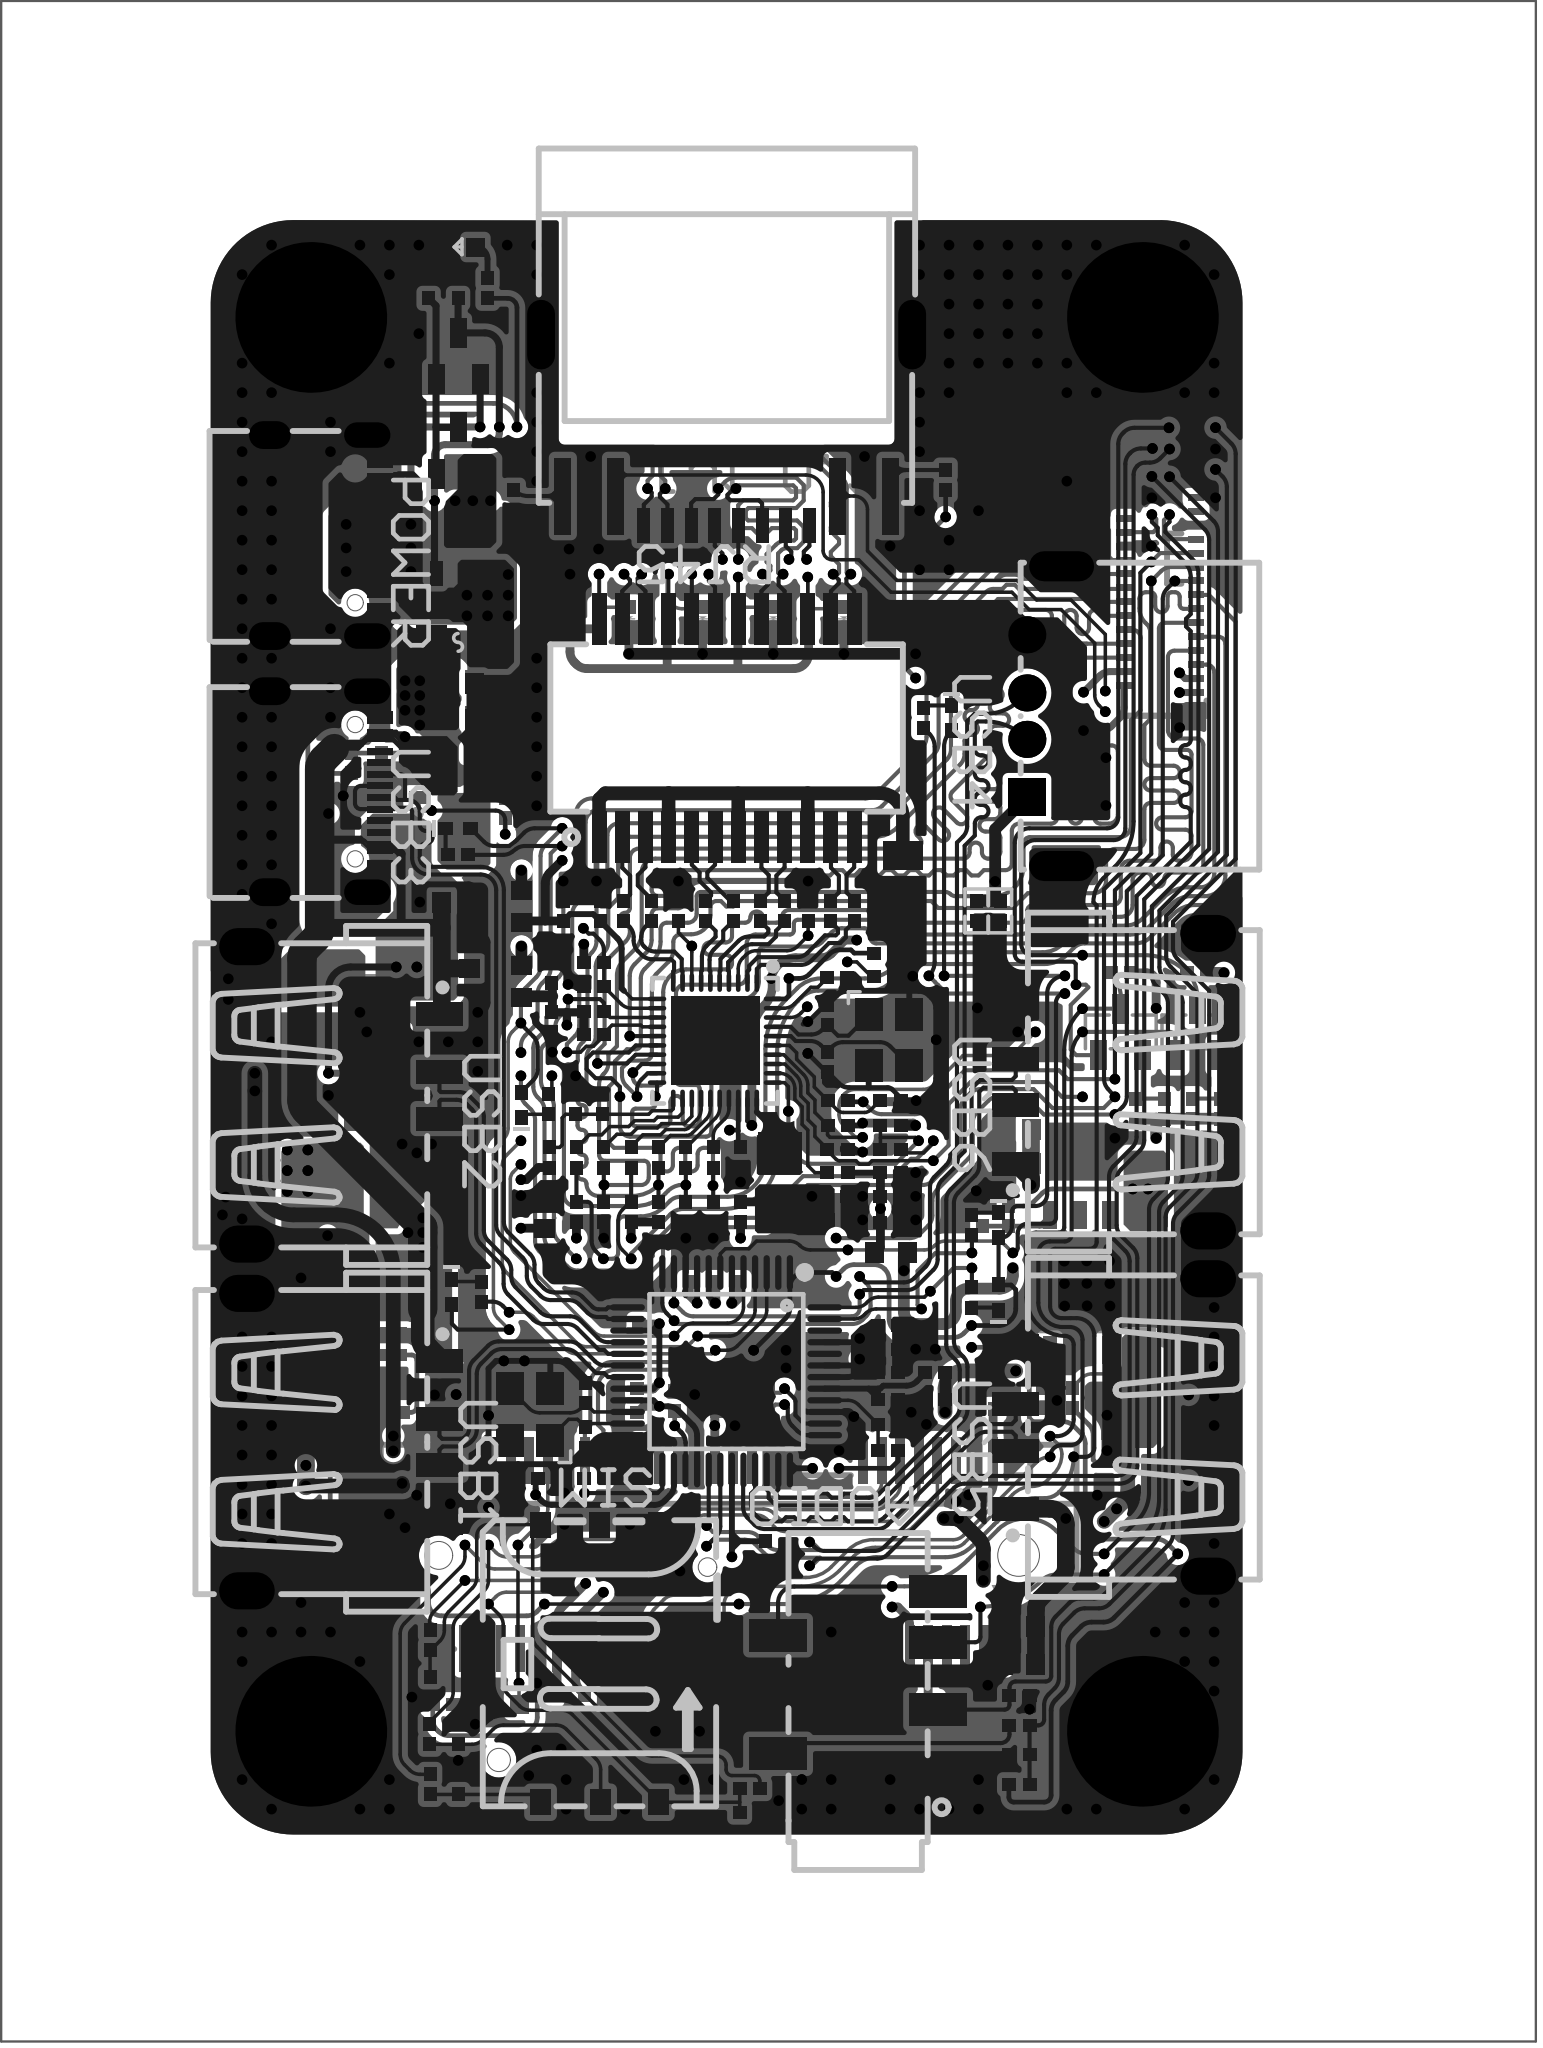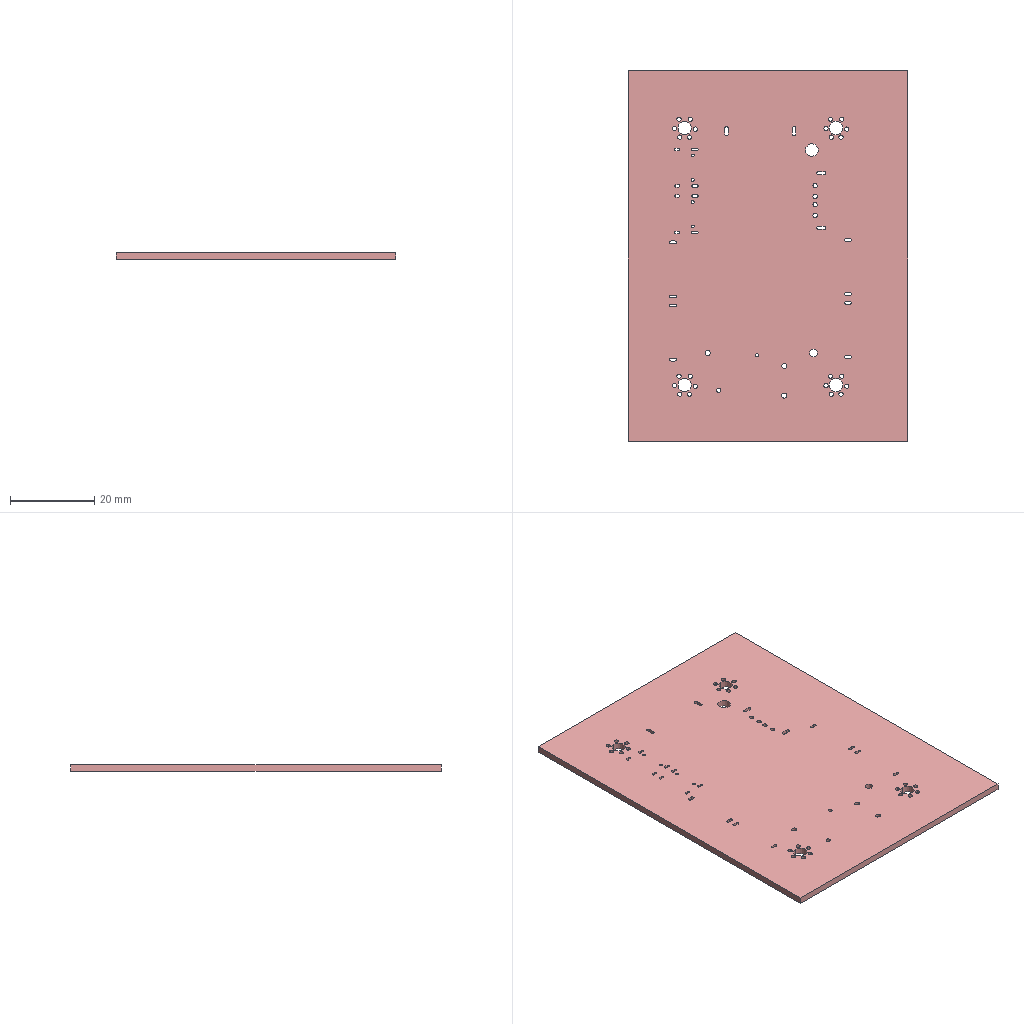Circuit board layout | Altium Designer | box 66.2 x 87.8 x 1.6 mm
Layer stack:
# Altium Designer layer stack of  (unit mm; dielectric type: 0 none, 1 core, 2 prepreg, 3 surface material)
index,name,kind,layer,copper_thickness_mm,dielectric_type,dielectric_thickness_mm,dielectric_material,dielectric_constant
0,Top Paste Mask Layer,other,,,,,,
1,Top Silkscreen Layer,other,,,,,,
2,Top Solder Mask Layer,dielectric,,,3,0,,0
3,Top Layer,copper,Top Layer,0.035,,,,
4,Dielectric1,dielectric,,,3,0.2104,7628 RC49% 8.6mil,0
5,GND,copper,GND,0.0152,,,,
6,Dielectric2,dielectric,,,3,1.065,1.1mm H/HOZ \u00BA\u00AC\u00CD\u00AD,0
7,VCC,copper,VCC,0.0152,,,,
8,Dielectric3,dielectric,,,3,0.2104,7628 RC49% 8.6mil,0
9,Bottom Layer,copper,Bottom Layer,0.035,,,,
10,Bottom Solder Mask Layer,dielectric,,,3,0,,0
11,Bottom Silkscreen Layer,other,,,,,,
12,Bottom Paste Mask Layer,other,,,,,,
# drill layer pairs: low layer,high layer
drill_pair,Top Layer,Bottom Layer
Part placement:
Designator,Comment,Layer,Footprint,Center-X(mm),Center-Y(mm),Rotation
R67,10kΩ,BottomLayer,R0402,118.125,115.839,0
R66,4.7kΩ,BottomLayer,R0402,118.76,109.997,90
R72,4.7kΩ,BottomLayer,R0402,121.203,109.997,270
FPC1,AFE03-S39FMA-1H,BottomLayer,fpc-smd_p0.30-39p_fgs-xj-h1.0,119.819,133.606,270
R70,10kΩ,BottomLayer,R0402,88.892,84.358,180
Q1,CJ2301 S1,TopLayer,SOT-23-3_L3.0-W1.7-P0.95-LS2.9-BR,89.55,134.127,270
C2,100nF,TopLayer,r0603,89.55,126.761,180
Q2,MMBT5401,TopLayer,SOT-23-3_L2.9-W1.3-P1.90-LS2.4-BR,89.55,138.315,270
Q3,MMBT5401,TopLayer,SOT-23-3_L2.9-W1.3-P1.90-LS2.4-BR,89.55,142.382,270
R6,50kΩ,TopLayer,R0402,89.55,145.303,270
R5,10kΩ,TopLayer,R0402,88.28,145.303,270
C1,10uF,TopLayer,r0603,89.55,128.285,180
F1,BSMD0805L-200,TopLayer,F0805,89.55,130.063,180
U1,MD7672B50SF4,BottomLayer,ESOP-8_L4.9-W3.9-P1.27-LS6.0-BL-EP,116.982,102.504,180
C3,4.7uF,BottomLayer,C0603,118.252,107.584,0
C4,4.7uF,BottomLayer,C0603,117.998,97.678,0
R74,10kΩ,TopLayer,R0402,113.758,80.914,180
R1,220kΩ,BottomLayer,R0402,116.043,97.551,270
R2,15kΩ,BottomLayer,R0402,113.299,105.373,90
R3,10kΩ,BottomLayer,R0402,112.156,105.373,270
R4,50kΩ,BottomLayer,R0402,114.747,97.551,90
U2,SY8113BADC,BottomLayer,TSOT-23-6_L2.9-W1.6-P0.95-LS2.8-BR,89.042,124.348,180
C8,100nF,BottomLayer,r0603,89.548,128.412,180
C6,100nF,BottomLayer,R0402,91.582,122.951,270
C9,22pF,BottomLayer,R0402,84.96,124.856,270
R8,232kΩ,BottomLayer,R0402,83.708,124.856,270
LED1,19-217/GHC-YR1S2/3T,TopLayer,LED0603-RD,89.5,147.075,0
R11,50kΩ,BottomLayer,R0402,86.248,124.856,90
C10,22uF,BottomLayer,r0603,89.548,117.744,180
C11,100nF,BottomLayer,r0603,89.548,119.268,180
C7,10uF,BottomLayer,r0603,89.548,126.888,180
R7,15kΩ,BottomLayer,R0402,91.582,124.856,270
R9,10kΩ,BottomLayer,R0402,91.582,126.761,270
R10,4.7kΩ,TopLayer,R0402,90.82,145.303,270
U4,RTL8211F-CG,TopLayer,WQFN-40_L5.0-W5.0-P0.4-BL-EP,100.629,112.918,180
L4,CBM160808U121T,TopLayer,L0603,92.281,115.465,90
Q4,SS8050,BottomLayer,SOT-23-3_L2.9-W1.3-P1.90-LS2.4-BR,118.125,113.299,270
L5,CBM160808U121T,TopLayer,L0603,108.218,103.787,0
L6,CBM160808U121T,TopLayer,L0603,92.281,118.697,90
R36,4.7kΩ,TopLayer,R0402,108.194,109.273,0
R33,0Ω,TopLayer,R0402,108.194,108.257,0
R19,4.7kΩ,TopLayer,R0402,105.912,109.273,0
R17,4.7kΩ,TopLayer,R0402,105.909,108.257,0
R14,4.7kΩ,TopLayer,R0402,105.911,107.241,0
Q5,SS8050,BottomLayer,SOT-23-3_L2.9-W1.3-P1.90-LS2.4-BR,121.427,113.299,270
R49,0Ω,TopLayer,R0402,93.474,107.895,270
U6,SMTWE2050MTJ,BottomLayer,SMD_BD4.4-L4.4-D2.8,113.317,138.831,180
R18,4.7kΩ,TopLayer,R0402,94.654,105.552,90
R16,4.7kΩ,TopLayer,R0402,97.012,105.552,90
R13,4.7kΩ,TopLayer,R0402,98.191,105.552,90
R21,4.7kΩ,TopLayer,R0402,95.405,114.188,0
R20,4.7kΩ,TopLayer,R0402,95.405,113.191,0
R30,4.7kΩ,TopLayer,R0402,99.371,105.552,90
R26,4.7kΩ,TopLayer,R0402,100.55,105.552,90
R22,4.7kΩ,TopLayer,R0402,95.833,105.552,90
R42,10kΩ,TopLayer,R0402,95.405,116.284,180
R73,0Ω,TopLayer,R0402,113.758,84.724,0
R41,22Ω,TopLayer,R0402,100.55,107.895,270
R43,22Ω,TopLayer,R0402,99.371,107.895,270
R44,22Ω,TopLayer,R0402,98.191,107.895,270
R45,22Ω,TopLayer,R0402,97.012,107.895,270
R46,22Ω,TopLayer,R0402,95.833,107.895,270
R48,22Ω,TopLayer,R0402,94.654,107.895,270
R28,100Ω,TopLayer,R0402,105.915,110.365,0
R23,120Ω,TopLayer,R0402,108.194,110.365,0
USB2,TYPE-C 16PIN 2MD(073),TopLayer,USB-C-SMD_TYPE-C-6PIN-2MD-073,83.81,123.637,270
R15,2.49kΩ,TopLayer,R0402,105.908,115.648,0
R50,0Ω,TopLayer,R0402,101.729,105.552,270
L3,G2406S,TopLayer,SMD-24_L15.1-W7.1-P1.00-LS10.0-BL,101.129,126.38,0
RJ1,RC01812,TopLayer,RJ45-TH_RC01812,101.129,139.207,0
R51,510Ω,TopLayer,R0402,110.57,137.048,90
R47,510Ω,TopLayer,R0402,91.951,137.048,270
R37,75Ω,BottomLayer,R0402,104.663,131.079,90
R38,75Ω,BottomLayer,R0402,101.615,131.079,90
R39,75Ω,BottomLayer,R0402,98.567,131.079,90
R40,75Ω,BottomLayer,R0402,95.646,131.079,90
D1,KLXES15AAA1,BottomLayer,D0402-BI,96.916,131.075,270
D2,KLXES15AAA1,BottomLayer,D0402-BI,100.091,131.075,270
D3,KLXES15AAA1,BottomLayer,D0402-BI,103.139,131.075,270
D4,KLXES15AAA1,BottomLayer,D0402-BI,106.187,131.075,270
R24,0Ω,TopLayer,R0402,96.696,118.506,90
R25,0Ω,TopLayer,R0402,97.873,118.506,90
R27,0Ω,TopLayer,R0402,100.229,118.506,90
R29,0Ω,TopLayer,R0402,101.407,118.506,90
R31,0Ω,TopLayer,R0402,102.584,118.506,90
R32,0Ω,TopLayer,R0402,103.635,118.506,90
R34,0Ω,TopLayer,R0402,105.609,118.506,90
R35,0Ω,TopLayer,R0402,106.66,118.506,90
USB1,TYPE-C 16PIN 2MD(073),TopLayer,USB-C-SMD_TYPE-C-6PIN-2MD-073,83.81,134.66,270
U5,FE2.1-CQFP48A,TopLayer,LQFP-48_L7.0-W7.0-P0.50-LS9.0-BL,101.107,98.694,180
R71,10kΩ,BottomLayer,R0402,121.427,115.839,180
LED7,XL-1005UGC,TopLayer,LED0402-RD_GREEN,112.855,104.981,270
LED6,XL-1005UGC,TopLayer,LED0402-RD_GREEN,112.855,101.869,90
LED5,XL-1005UGC,TopLayer,LED0402-RD_GREEN,110.823,126.81,270
LED4,XL-1005UGC,TopLayer,LED0402-RD_GREEN,89.55,122.062,0
LED3,XL-1005UGC,TopLayer,LED0402-RD_GREEN,92.268,110.162,90
LED2,XL-1005UGC,TopLayer,LED0402-RD_GREEN,89.283,102.123,270
X2,12MHz,TopLayer,OSC-SMD_4P-L3.2-W2.5-BL,92.652,96.836,90
R58,2.7kΩ,BottomLayer,R0402,98.89,97.402,90
R60,47kΩ,TopLayer,R0402,110.133,98.63,0
R61,100kΩ,TopLayer,R0402,108.092,97.487,180
R59,100kΩ,TopLayer,R0402,108.092,95.28,0
USB4,AF 10.0 HC6.3,TopLayer,USB-A-TH_AF-10.0-HC6.3,114.823,126.888,90
C48,10uF,TopLayer,r0603,93.294,105.552,270
CN1,1775862-2,BottomLayer,PCI-SMD_1775862-2,101.218,90.62,0
R63,0Ω,TopLayer,R0402,88.335,83.073,270
R64,0Ω,TopLayer,R0402,88.344,80.914,270
D5,KLXES15AAA1,TopLayer,R0402,89.555,80.914,90
LED8,19-217/GHC-YR1S2/3T,BottomLayer,LED0603-RD,91.378,84.338,180
L7,CBG160808U000T,BottomLayer,L0603,110.632,84.334,180
R68,2.2Ω,BottomLayer,R0402,102.496,96.957,0
R69,2.2Ω,BottomLayer,R0402,102.496,97.998,0
AUDIO1,PJ-393,TopLayer,AUDIO-SMD_PJ-393,106.797,85.232,0
R75,1kΩ,TopLayer,R0402,113.758,83.454,180
K1,,TopLayer,125_X_300,83.263,83.159,0
K2,,TopLayer,125_X_300,119.121,83.159,0
K3,,TopLayer,125_X_300,83.263,144.008,0
K4,,TopLayer,125_X_300,119.121,144.008,0
U7,SY6280AAC,BottomLayer,SOT-23-5_L3.0-W1.7-P0.95-LS2.8-BL,85.613,100.345,270
R76,NC,BottomLayer,R0805,85.867,103.52,0
R77,10kΩ,BottomLayer,R0402,84.47,96.964,180
R78,10kΩ,BottomLayer,R0402,86.756,96.927,0
C75,10uF,BottomLayer,C0603,89.55,105.171,180
C74,100nF,BottomLayer,C0603,89.55,103.139,180
C72,100nF,BottomLayer,C0603,85.74,107.33,0
C73,1uF,BottomLayer,C0603,85.74,105.552,180
C63,10uF,BottomLayer,r0603,113.553,107.647,0
C62,100nF,BottomLayer,r0603,113.553,109.108,0
C65,10uF,TopLayer,r0603,113.766,87.709,0
C64,100nF,TopLayer,r0603,113.766,86.058,0
C67,10uF,BottomLayer,r0603,89.55,101.361,180
C66,100nF,BottomLayer,r0603,89.55,99.71,180
C69,10uF,TopLayer,r0603,89.55,118.887,180
C68,100nF,TopLayer,r0603,90.058,116.728,270
C71,10uF,TopLayer,r0603,89.55,123.967,180
C70,100nF,TopLayer,r0603,89.55,125.364,180
CN2,908-161A2021S10110,TopLayer,USB-A-SMD_AF-SMT-SHORT,84.597,95.646,270
CN5,908-161A2021S10110,TopLayer,USB-A-SMD_AF-SMT-SHORT,117.744,111.135,90
CN3,908-161A2021S10110,TopLayer,USB-A-SMD_AF-SMT-SHORT,84.597,110.569,270
CN4,908-161A2021S10110,TopLayer,USB-A-SMD_AF-SMT-SHORT,117.744,96.276,90
CARD1,SMN-304,TopLayer,SIM-SMD_SMN-304,95.646,86.121,0
D7,KLXES15AAA1,TopLayer,R0402,102.123,79.707,0
D6,KLXES15AAA1,TopLayer,R0402,89.55,83.073,90
R62,15kΩ,TopLayer,R0402,102.126,80.72,180
R65,0Ω,TopLayer,R0402,88.342,87.137,90
D8,KLXES15AAA1,TopLayer,R0402,88.342,85.105,270
C13,4.7uF,BottomLayer,r0603,82.565,114.188,90
R12,10kΩ,BottomLayer,R0603,85.74,111.521,0
C15,100nF,BottomLayer,C0603,85.74,109.489,180
C14,100nF,BottomLayer,C0603,80.787,114.188,90
U3,TP5108E23E-18,BottomLayer,SOT-23-5_L3.0-W1.7-P0.95-LS2.8-BL,85.613,114.188,270
C12,10uF,BottomLayer,r0603,89.55,115.204,180
X1,25MHz,TopLayer,OSC-SMD_4P-L3.2-W2.5-BL,108.13,112.956,270
R52,4.7kΩ,TopLayer,R0402,90.557,102.123,270
R53,4.7kΩ,TopLayer,R0402,93.468,110.188,90
R54,4.7kΩ,TopLayer,R0402,89.55,120.919,0
R55,4.7kΩ,TopLayer,R0402,109.609,126.825,270
R56,4.7kΩ,TopLayer,R0402,111.705,101.869,90
R57,4.7kΩ,TopLayer,R0402,111.705,104.981,270
L1,2.2uH,BottomLayer,IND-SMD_L2.5-W2.0_WPN252012H,88.661,121.427,0
L2,2.2uH,TopLayer,IND-SMD_L2.5-W2.0_WPN252012H,103.428,106.885,90
C5,100nF,BottomLayer,R0402,117.99,96.027,0
C23,100nF,TopLayer,R0402,93.563,115.839,270
C31,100nF,TopLayer,R0402,108.194,105.082,180
C30,100nF,TopLayer,R0402,108.194,106.225,180
C29,100nF,TopLayer,R0402,108.194,107.241,180
C34,100nF,TopLayer,R0402,107.937,116.69,180
C33,100nF,TopLayer,R0402,95.67,118.506,270
C32,100nF,TopLayer,R0402,94.084,118.506,270
C18,100nF,TopLayer,R0402,105.908,106.225,180
C19,4.7uF,TopLayer,R0402,105.914,105.209,180
C24,100nF,TopLayer,R0402,94.617,110.188,270
C27,100nF,TopLayer,R0402,99.051,118.506,270
C26,100nF,TopLayer,R0402,104.643,118.506,270
C28,100nF,TopLayer,R0402,107.937,115.699,180
C17,100nF,TopLayer,R0402,101.729,107.895,90
C16,100nF,TopLayer,R0402,93.563,113.709,90
C22,100nF,TopLayer,R0402,95.405,115.267,0
C25,100nF,TopLayer,R0402,95.797,110.188,270
C21,1nF,BottomLayer,R0402,94.376,131.079,270
CX1,12pF,TopLayer,R0402,105.462,114.036,270
CX2,12pF,TopLayer,R0402,105.47,112.016,90
C43,100nF,TopLayer,R0402,110.133,97.487,0
C44,100nF,TopLayer,R0402,108.092,96.408,180
C35,100nF,BottomLayer,R0402,96.853,97.932,0
C36,100nF,BottomLayer,R0402,99.519,102.948,270
C37,100nF,TopLayer,R0402,108.092,99.647,180
C38,100nF,TopLayer,R0402,108.092,98.63,180
C39,100nF,TopLayer,R0402,92.562,94.058,0
C40,100nF,TopLayer,R0402,102.822,90.947,90
C41,100nF,BottomLayer,R0402,96.916,100.726,0
C42,100nF,TopLayer,R0402,108.092,100.662,180
C45,100nF,TopLayer,R0402,94.568,94.058,0
C46,100nF,BottomLayer,R0402,96.853,96.916,0
C47,100nF,BottomLayer,R0402,101.678,102.948,270
C49,100nF,BottomLayer,R0402,100.599,102.948,270
C51,12pF,TopLayer,R0402,95.047,97.742,90
C50,12pF,TopLayer,R0402,95.047,95.844,90
C52,100nF,BottomLayer,R0402,100.268,96.953,0
C53,100nF,BottomLayer,R0402,112.675,97.487,270
C54,100nF,BottomLayer,R0402,88.988,96.927,0
C55,100nF,BottomLayer,R0402,95.011,84.343,90
C56,100nF,BottomLayer,R0402,93.614,84.343,90
C59,100nF,TopLayer,R0402,113.758,82.184,180
C20,10nF,TopLayer,r1206,108.727,119.395,90
C57,1nF,BottomLayer,r0402,120,109.997,90
C58,1nF,BottomLayer,r0402,122.443,109.997,270
C61,10uF,TopLayer,R0402,111.902,118.506,90
C60,100nF,TopLayer,R0402,112.918,118.506,90
Pad and via stacks:
# Altium Designer via and pad stacks of  (unit mm). Each distinct definition once, with the count of objects using it.
# via: kind,start_layer,end_layer,hole_mm,diameter_mm,mode(0 simple;1 top-mid-bottom;2 full stack),diameter_per_layer,count,example_net
# pad: kind,layer,hole_mm,hole_type(0 round;1 square;2 slot),plating,top_size,top_shape(1 round;2 rect;3 octagon;9 rounded rect),mid_size,bottom_size,mode,footprint,size_per_layer,count,example
pad,Bottom Layer,0,0,plated,0.5657x0.54,2,0.5657x0.54,0.5657x0.54,0,R0402,,78,R67.2
pad,Bottom Layer,0,0,plated,0.3x0.65,2,0.3x0.65,0.3x0.65,0,fpc-smd_p0.30-39p_fgs-xj-h1.0,,39,FPC1.1
pad,Bottom Layer,0,0,plated,0.4x0.95,2,0.4x0.95,0.4x0.95,0,fpc-smd_p0.30-39p_fgs-xj-h1.0,,2,FPC1.40
pad,Bottom Layer,0,0,plated,0.6x1.2,2,0.6x1.2,0.6x1.2,0,ESOP-8_L4.9-W3.9-P1.27-LS6.0-BL-EP,,8,U1.1
pad,Bottom Layer,0,0,plated,3.3x2.4,2,3.3x2.4,3.3x2.4,0,ESOP-8_L4.9-W3.9-P1.27-LS6.0-BL-EP,,1,U1.9
pad,Bottom Layer,0,0,plated,0.8x0.9,2,0.8x0.9,0.8x0.9,0,C0603,,16,C3.2
pad,Bottom Layer,0,0,plated,0.8x0.532,2,0.8x0.532,0.8x0.532,0,TSOT-23-6_L2.9-W1.6-P0.95-LS2.8-BR,,6,U2.6
pad,Bottom Layer,0,0,plated,0.8x0.9,2,0.8x0.9,0.8x0.9,0,r0603,,20,C8.1
pad,Bottom Layer,0,0,plated,1.25x0.7,2,1.25x0.7,1.25x0.7,0,SOT-23-3_L2.9-W1.3-P1.90-LS2.4-BR,,6,Q4.1
pad,Bottom Layer,0,0,plated,0.2292x0.2292,1,0.2292x0.2292,0.2292x0.2292,0,SMD_BD4.4-L4.4-D2.8,,4,U6.1
pad,Bottom Layer,0,0,plated,0.6x0.6,2,0.6x0.6,0.6x0.6,0,D0402-BI,,8,D1.1
pad,Bottom Layer,0,0,plated,2.4x3.4,2,2.4x3.4,2.4x3.4,0,PCI-SMD_1775862-2,,2,CN1.53
pad,Bottom Layer,0,0,plated,0.4x2,2,0.4x2,0.4x2,0,PCI-SMD_1775862-2,,51,CN1.52
pad,Bottom Layer,0,0,plated,0.4x1.2,2,0.4x1.2,0.4x1.2,0,PCI-SMD_1775862-2,,1,CN1.15
pad,Bottom Layer,0,0,plated,0.8x0.8,2,0.8x0.8,0.8x0.8,0,LED0603-RD,,2,LED8.2
pad,Bottom Layer,0,0,plated,0.8x0.864,2,0.8x0.864,0.8x0.864,0,L0603,,2,L7.1
pad,Bottom Layer,0,0,plated,0.49x1.175,2,0.49x1.175,0.49x1.175,0,SOT-23-5_L3.0-W1.7-P0.95-LS2.8-BL,,4,U7.5
pad,Bottom Layer,0,0,plated,0.49x1.157,2,0.49x1.157,0.49x1.157,0,SOT-23-5_L3.0-W1.7-P0.95-LS2.8-BL,,6,U7.1
pad,Bottom Layer,0,0,plated,1.133x1.377,2,1.133x1.377,1.133x1.377,0,R0805,,2,R76.2
pad,Bottom Layer,0,0,plated,0.8065x0.864,2,0.8065x0.864,0.8065x0.864,0,R0603,,2,R12.2
pad,Bottom Layer,0,0,plated,1.724x1.87,2,1.724x1.87,1.724x1.87,0,IND-SMD_L2.5-W2.0_WPN252012H,,2,L1.1
pad,Top Layer,0,0,plated,1.038x0.532,2,1.038x0.532,1.038x0.532,0,SOT-23-3_L3.0-W1.7-P0.95-LS2.9-BR,,3,Q1.3
pad,Top Layer,0,0,plated,0.8x0.9,2,0.8x0.9,0.8x0.9,0,r0603,,18,C2.2
pad,Top Layer,0,0,plated,1.25x0.7,2,1.25x0.7,1.25x0.7,0,SOT-23-3_L2.9-W1.3-P1.90-LS2.4-BR,,6,Q2.3
pad,Top Layer,0,0,plated,0.5657x0.54,2,0.5657x0.54,0.5657x0.54,0,R0402,,180,R6.2
pad,Top Layer,0,0,plated,1.335x1.5,2,1.335x1.5,1.335x1.5,0,F0805,,2,F1.1
pad,Top Layer,0,0,plated,0.8x0.8,2,0.8x0.8,0.8x0.8,0,LED0603-RD,,2,LED1.2
pad,Top Layer,0,0,plated,3.8x3.8,2,3.8x3.8,3.8x3.8,0,WQFN-40_L5.0-W5.0-P0.4-BL-EP,,1,U4.41
pad,Top Layer,0,0,plated,0.2x0.8,1,0.2x0.8,0.2x0.8,0,WQFN-40_L5.0-W5.0-P0.4-BL-EP,,40,U4.1
pad,Top Layer,0,0,plated,0.8x0.864,2,0.8x0.864,0.8x0.864,0,L0603,,6,L4.1
pad,Top Layer,0,0,plated,0.55x1.1,2,0.55x1.1,0.55x1.1,0,USB-C-SMD_TYPE-C-6PIN-2MD-073,,8,USB2.1
pad,Top Layer,0,0,plated,0.3x1.1,2,0.3x1.1,0.3x1.1,0,USB-C-SMD_TYPE-C-6PIN-2MD-073,,16,USB2.3
pad,Top Layer,0,0,plated,0.64x2.2,2,0.64x2.2,0.64x2.2,0,SMD-24_L15.1-W7.1-P1.00-LS10.0-BL,,24,L3.1
pad,Top Layer,0,0,plated,0.7x3.3,2,0.7x3.3,0.7x3.3,0,RJ45-TH_RC01812,,4,RJ1.12
pad,Top Layer,0,0,plated,0.55x1.5,2,0.55x1.5,0.55x1.5,0,RJ45-TH_RC01812,,8,RJ1.8
pad,Top Layer,0,0,plated,0.27x1.5,1,0.27x1.5,0.27x1.5,0,LQFP-48_L7.0-W7.0-P0.50-LS9.0-BL,,24,U5.1
pad,Top Layer,0,0,plated,1.5x0.27,1,1.5x0.27,1.5x0.27,0,LQFP-48_L7.0-W7.0-P0.50-LS9.0-BL,,24,U5.13
pad,Top Layer,0,0,plated,0.6365x0.54,2,0.6365x0.54,0.6365x0.54,0,LED0402-RD_GREEN,,12,LED7.2
pad,Top Layer,0,0,plated,1.4x1.2,2,1.4x1.2,1.4x1.2,0,OSC-SMD_4P-L3.2-W2.5-BL,,8,X2.1
pad,Top Layer,0,0,plated,2.5x1.4,2,2.5x1.4,2.5x1.4,0,AUDIO-SMD_PJ-393,,7,AUDIO1.4
pad,Top Layer,0,0,plated,2x1,2,2x1,2x1,0,USB-A-SMD_AF-SMT-SHORT,,16,CN2.4
pad,Top Layer,0,0,plated,0.9x1.1,2,0.9x1.1,0.9x1.1,0,SIM-SMD_SMN-304,,6,CARD1.C7
pad,Top Layer,0,0,plated,1x3.29,2,1x3.29,1x3.29,0,SIM-SMD_SMN-304,,2,CARD1.1
pad,Top Layer,0,0,plated,1.724x1.87,2,1.724x1.87,1.724x1.87,0,IND-SMD_L2.5-W2.0_WPN252012H,,2,L2.1
pad,Top Layer,0,0,plated,1.208x1.701,2,1.208x1.701,1.208x1.701,0,r1206,,2,C20.2
pad,Multi-Layer,0.6,2,plated,1.1x2,1,1.1x2,1.1x2,0,USB-C-SMD_TYPE-C-6PIN-2MD-073,,4,USB2.13
pad,Multi-Layer,0.6,2,plated,1.2x1.8,1,1.2x1.8,1.2x1.8,0,USB-C-SMD_TYPE-C-6PIN-2MD-073,,4,USB2.13
pad,Multi-Layer,0.8,2,plated,1.2x3,1,1.2x3,1.2x3,0,RJ45-TH_RC01812,,2,RJ1.14
pad,Multi-Layer,0.8,2,plated,1.3x2.8,1,1.3x2.8,1.3x2.8,0,USB-A-TH_AF-10.0-HC6.3,,2,USB4.6
pad,Multi-Layer,1,0,plated,1.6x1.6,1,1.6x1.6,1.6x1.6,0,USB-A-TH_AF-10.0-HC6.3,,3,USB4.4
pad,Multi-Layer,1,0,plated,1.6x1.6,2,1.6x1.6,1.6x1.6,0,USB-A-TH_AF-10.0-HC6.3,,1,USB4.1
pad,Multi-Layer,1.016,2,plated,1.016x1.016,1,1.016x1.016,1.016x1.016,0,125 X 300,,24,K1.1
pad,Multi-Layer,3.175,2,plated,6.5x6.5,1,6.5x6.5,6.5x6.5,0,125 X 300,,4,K1.1
pad,Multi-Layer,0.7,2,plated,2.4x1.6,1,2.4x1.6,2.4x1.6,0,USB-A-SMD_AF-SMT-SHORT,,8,CN2.SH1
via,Top Layer,Bottom Layer,0.254,0.4572,0,,529,GMAC0_MDC
Copper pours:
name,layer,net,type(0 solid;1 hatched;2 none)
Top Layer-VCC5V0_USB_VBUS,Top Layer,VCC5V0_USB_VBUS,0
Top Layer-VCC5V0_SYS,Top Layer,VCC5V0_SYS,0
Top Layer-IN_5V,Top Layer,IN_5V,0
Top Layer-GND,Top Layer,GND,0
Top Layer-LDO_OUT,Top Layer,LDO_OUT,0
Top Layer-1V05_PHY,Top Layer,1V05_PHY,0
Top Layer-VCC5V0_USB_HOST,Top Layer,VCC5V0_USB_HOST,0
Top Layer-VCC3V3_USB,Top Layer,VCC3V3_USB,0
Bottom Layer-IN_5V,Bottom Layer,IN_5V,0
Bottom Layer-VCC_4G,Bottom Layer,VCC_4G,0
Bottom Layer-VCC5V0_USB_VBUS,Bottom Layer,VCC5V0_USB_VBUS,0
Bottom Layer-IN_5V 1,Bottom Layer,IN_5V,0
Bottom Layer-$5N2260,Bottom Layer,$5N2260,0
Bottom Layer-VCC3V3_SYS,Bottom Layer,VCC3V3_SYS,0
Bottom Layer-VCC1V8,Bottom Layer,VCC1V8,0
Bottom Layer-GND,Bottom Layer,GND,0
Bottom Layer-IN_5V 2,Bottom Layer,IN_5V,0
Bottom Layer-VCC5V0_USB_HOST,Bottom Layer,VCC5V0_USB_HOST,0
Bottom Layer-GND 1,Bottom Layer,GND,0
GND-GND,GND,GND,0
VCC-GND,VCC,GND,0
VCC-IN_5V,VCC,IN_5V,0
Design rules, without the lines most boards share:
# Altium Designer design rules of  (exported by Altium Designer, unit mm)
# columns: name | kind | enabled | priority | scope1 | scope2 | descriptor | typed fields (field=value)
copperThickness2oz | 0 | disabled | 1 | All | All | Clearance Constraint (Gap=6mil) (Disabled)(All),(All) | gap=0.1524
Plane_innerPlane | 0 | disabled | 2 | All | All | Clearance Constraint (Gap=6mil) (Disabled)(All),(All) | gap=0.1524
Copper_copperRegion | 0 | disabled | 3 | All | All | Clearance Constraint (Gap=6mil) (Disabled)(All),(All) | gap=0.1524
copperThickness1oz | 0 | enabled | 4 | All | All | Clearance Constraint (Gap=6mil) (All),(All) | gap=0.1524
otherClearance | 52 | enabled | 1 | All | All | Hole To Hole Clearance (Gap=11.8mil) (All),(All) | gap=0.2997
copperThickness1oz_2 | 2 | enabled | 2 | All | All | Width Constraint (Min=5mil) (Max=100mil) (Preferred=7mil) (All) |
differentialPair | 51 | enabled | 1 | All | All | Differential Pairs Uncoupled Length using the Gap Constraints (Min=6mil) (Max=6mil) (Prefered=6mil)  and Width Constraints (Min=7mil) (Max=7mil) (Prefered=7mil) (All) |
viaSize | 11 | enabled | 1 | All | All | Routing Via (MinHoleWidth=10mil) (MaxHoleWidth=10mil) (PreferredHoleWidth=10mil) (MinWidth=18mil) (MaxWidth=18mil) (PreferedWidth=18mil) (All) | via_min_hole=0.254 via_max_hole=0.254 via_preferred_diameter=0.4572 via_preferred_hole=0.254
copperRegion | 20 | enabled | 1 | All | All | Polygon Connect Rule(Direct Connect )(Conductor Width=10mil) (Relief Angle=90 Angle) (Entries=4) (Air Gap Width=10mil) (All),(All) | connect_style(0=relief,1=direct,2=none)=1 relief_conductor_width=0.254 relief_entries=4